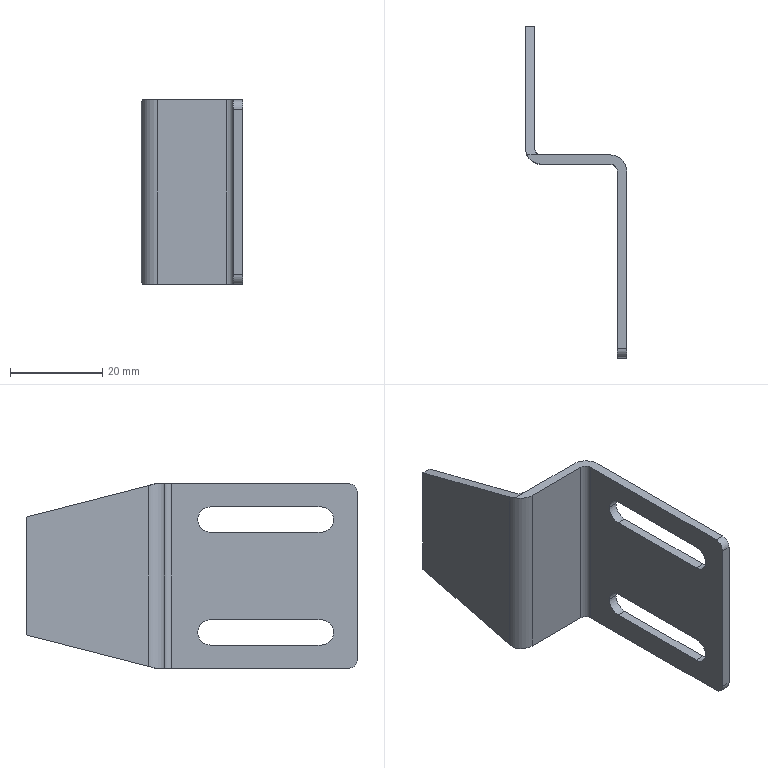Part | NX | features BREP 1 | 1 solid | 28 faces | box 22 x 72 x 40 mm | volume 6159 mm3 | plane 16 | cylinder 12 | commonest cylinder face diameters 5.5 x6 3 x2 4 x2 7 x2
STEP:
#1=CARTESIAN_POINT('',(0.,-7.25,-12.25));
#2=VERTEX_POINT('',#1);
#3=CARTESIAN_POINT('',(0.,-10.,-9.5));
#4=VERTEX_POINT('',#3);
#5=CARTESIAN_POINT('',(0.,-10.,-12.25));
#6=DIRECTION('',(1.,0.,0.));
#7=DIRECTION('',(0.,1.,0.));
#8=AXIS2_PLACEMENT_3D('',#5,#6,#7);
#9=CIRCLE('',#8,2.75);
#10=EDGE_CURVE('',#2,#4,#9,.T.);
#11=ORIENTED_EDGE('',*,*,#10,.F.);
#12=CARTESIAN_POINT('',(2.,-7.25,-12.25));
#13=VERTEX_POINT('',#12);
#14=CARTESIAN_POINT('',(-20.,-7.25,-12.25));
#15=DIRECTION('',(1.,0.,0.));
#16=VECTOR('',#15,1000.);
#17=LINE('',#14,#16);
#18=EDGE_CURVE('',#2,#13,#17,.T.);
#19=ORIENTED_EDGE('',*,*,#18,.T.);
#20=CARTESIAN_POINT('',(2.,-10.,-9.5));
#21=VERTEX_POINT('',#20);
#22=CARTESIAN_POINT('',(2.,-10.,-12.25));
#23=DIRECTION('',(1.,0.,0.));
#24=DIRECTION('',(0.,-1.,0.));
#25=AXIS2_PLACEMENT_3D('',#22,#23,#24);
#26=CIRCLE('',#25,2.75);
#27=EDGE_CURVE('',#13,#21,#26,.T.);
#28=ORIENTED_EDGE('',*,*,#27,.T.);
#29=CARTESIAN_POINT('',(-20.,-10.,-9.5));
#30=DIRECTION('',(1.,0.,0.));
#31=VECTOR('',#30,1000.);
#32=LINE('',#29,#31);
#33=EDGE_CURVE('',#4,#21,#32,.T.);
#34=ORIENTED_EDGE('',*,*,#33,.F.);
#35=EDGE_LOOP('',(#11,#19,#28,#34));
#36=FACE_BOUND('',#35,.T.);
#37=CARTESIAN_POINT('',(-20.,-10.,-12.25));
#38=DIRECTION('',(1.,0.,0.));
#39=DIRECTION('',(0.,1.,0.));
#40=AXIS2_PLACEMENT_3D('',#37,#38,#39);
#41=CYLINDRICAL_SURFACE('',#40,2.75);
#42=ADVANCED_FACE('',(#36),#41,.F.);
#43=CARTESIAN_POINT('',(0.,-7.25,12.25));
#44=VERTEX_POINT('',#43);
#45=CARTESIAN_POINT('',(0.,-10.,15.));
#46=VERTEX_POINT('',#45);
#47=CARTESIAN_POINT('',(0.,-10.,12.25));
#48=DIRECTION('',(1.,0.,0.));
#49=DIRECTION('',(0.,1.,0.));
#50=AXIS2_PLACEMENT_3D('',#47,#48,#49);
#51=CIRCLE('',#50,2.75);
#52=EDGE_CURVE('',#44,#46,#51,.T.);
#53=ORIENTED_EDGE('',*,*,#52,.F.);
#54=CARTESIAN_POINT('',(2.,-7.25,12.25));
#55=VERTEX_POINT('',#54);
#56=CARTESIAN_POINT('',(-20.,-7.25,12.25));
#57=DIRECTION('',(1.,0.,0.));
#58=VECTOR('',#57,1000.);
#59=LINE('',#56,#58);
#60=EDGE_CURVE('',#44,#55,#59,.T.);
#61=ORIENTED_EDGE('',*,*,#60,.T.);
#62=CARTESIAN_POINT('',(2.,-10.,15.));
#63=VERTEX_POINT('',#62);
#64=CARTESIAN_POINT('',(2.,-10.,12.25));
#65=DIRECTION('',(1.,0.,0.));
#66=DIRECTION('',(0.,1.,0.));
#67=AXIS2_PLACEMENT_3D('',#64,#65,#66);
#68=CIRCLE('',#67,2.75);
#69=EDGE_CURVE('',#55,#63,#68,.T.);
#70=ORIENTED_EDGE('',*,*,#69,.T.);
#71=CARTESIAN_POINT('',(-20.,-10.,15.));
#72=DIRECTION('',(1.,0.,0.));
#73=VECTOR('',#72,1000.);
#74=LINE('',#71,#73);
#75=EDGE_CURVE('',#46,#63,#74,.T.);
#76=ORIENTED_EDGE('',*,*,#75,.F.);
#77=EDGE_LOOP('',(#53,#61,#70,#76));
#78=FACE_BOUND('',#77,.T.);
#79=CARTESIAN_POINT('',(-20.,-10.,12.25));
#80=DIRECTION('',(1.,0.,0.));
#81=DIRECTION('',(0.,1.,0.));
#82=AXIS2_PLACEMENT_3D('',#79,#80,#81);
#83=CYLINDRICAL_SURFACE('',#82,2.75);
#84=ADVANCED_FACE('',(#78),#83,.F.);
#85=CARTESIAN_POINT('',(2.,-42.,18.));
#86=VERTEX_POINT('',#85);
#87=CARTESIAN_POINT('',(2.,-42.,-18.));
#88=VERTEX_POINT('',#87);
#89=CARTESIAN_POINT('',(2.,-42.,20.));
#90=DIRECTION('',(0.,0.,-1.));
#91=VECTOR('',#90,1000.);
#92=LINE('',#89,#91);
#93=EDGE_CURVE('',#86,#88,#92,.T.);
#94=ORIENTED_EDGE('',*,*,#93,.T.);
#95=CARTESIAN_POINT('',(2.,-40.,-20.));
#96=VERTEX_POINT('',#95);
#97=CARTESIAN_POINT('',(2.,-40.,-18.));
#98=DIRECTION('',(1.,0.,0.));
#99=DIRECTION('',(0.,-1.,0.));
#100=AXIS2_PLACEMENT_3D('',#97,#98,#99);
#101=CIRCLE('',#100,2.);
#102=EDGE_CURVE('',#88,#96,#101,.T.);
#103=ORIENTED_EDGE('',*,*,#102,.T.);
#104=CARTESIAN_POINT('',(2.,-1.5,-20.));
#105=VERTEX_POINT('',#104);
#106=CARTESIAN_POINT('',(2.,2.,-20.));
#107=DIRECTION('',(0.,1.,0.));
#108=VECTOR('',#107,1000.);
#109=LINE('',#106,#108);
#110=EDGE_CURVE('',#96,#105,#109,.T.);
#111=ORIENTED_EDGE('',*,*,#110,.T.);
#112=CARTESIAN_POINT('',(2.,-1.5,20.));
#113=VERTEX_POINT('',#112);
#114=CARTESIAN_POINT('',(2.,-1.5,20.));
#115=DIRECTION('',(0.,0.,1.));
#116=VECTOR('',#115,1000.);
#117=LINE('',#114,#116);
#118=EDGE_CURVE('',#105,#113,#117,.T.);
#119=ORIENTED_EDGE('',*,*,#118,.T.);
#120=CARTESIAN_POINT('',(2.,-40.,20.));
#121=VERTEX_POINT('',#120);
#122=CARTESIAN_POINT('',(2.,2.,20.));
#123=DIRECTION('',(0.,1.,0.));
#124=VECTOR('',#123,1000.);
#125=LINE('',#122,#124);
#126=EDGE_CURVE('',#121,#113,#125,.T.);
#127=ORIENTED_EDGE('',*,*,#126,.F.);
#128=CARTESIAN_POINT('',(2.,-40.,18.));
#129=DIRECTION('',(1.,0.,0.));
#130=DIRECTION('',(0.,-1.,0.));
#131=AXIS2_PLACEMENT_3D('',#128,#129,#130);
#132=CIRCLE('',#131,2.);
#133=EDGE_CURVE('',#121,#86,#132,.T.);
#134=ORIENTED_EDGE('',*,*,#133,.T.);
#135=EDGE_LOOP('',(#94,#103,#111,#119,#127,#134));
#136=FACE_BOUND('',#135,.T.);
#137=CARTESIAN_POINT('',(2.,-34.,-9.5));
#138=VERTEX_POINT('',#137);
#139=CARTESIAN_POINT('',(2.,-10.,-9.5));
#140=DIRECTION('',(0.,-1.,0.));
#141=VECTOR('',#140,1000.);
#142=LINE('',#139,#141);
#143=EDGE_CURVE('',#21,#138,#142,.T.);
#144=ORIENTED_EDGE('',*,*,#143,.F.);
#145=ORIENTED_EDGE('',*,*,#27,.F.);
#146=CARTESIAN_POINT('',(2.,-10.,-15.));
#147=VERTEX_POINT('',#146);
#148=CARTESIAN_POINT('',(2.,-10.,-12.25));
#149=DIRECTION('',(1.,0.,0.));
#150=DIRECTION('',(0.,-1.,0.));
#151=AXIS2_PLACEMENT_3D('',#148,#149,#150);
#152=CIRCLE('',#151,2.75);
#153=EDGE_CURVE('',#147,#13,#152,.T.);
#154=ORIENTED_EDGE('',*,*,#153,.F.);
#155=CARTESIAN_POINT('',(2.,-34.,-15.));
#156=VERTEX_POINT('',#155);
#157=CARTESIAN_POINT('',(2.,-10.,-15.));
#158=DIRECTION('',(0.,1.,0.));
#159=VECTOR('',#158,1000.);
#160=LINE('',#157,#159);
#161=EDGE_CURVE('',#156,#147,#160,.T.);
#162=ORIENTED_EDGE('',*,*,#161,.F.);
#163=CARTESIAN_POINT('',(2.,-34.,-12.25));
#164=DIRECTION('',(1.,0.,0.));
#165=DIRECTION('',(0.,-1.,0.));
#166=AXIS2_PLACEMENT_3D('',#163,#164,#165);
#167=CIRCLE('',#166,2.75);
#168=EDGE_CURVE('',#138,#156,#167,.T.);
#169=ORIENTED_EDGE('',*,*,#168,.F.);
#170=EDGE_LOOP('',(#144,#145,#154,#162,#169));
#171=FACE_BOUND('',#170,.T.);
#172=CARTESIAN_POINT('',(2.,-34.,15.));
#173=VERTEX_POINT('',#172);
#174=CARTESIAN_POINT('',(2.,-10.,15.));
#175=DIRECTION('',(0.,-1.,0.));
#176=VECTOR('',#175,1000.);
#177=LINE('',#174,#176);
#178=EDGE_CURVE('',#63,#173,#177,.T.);
#179=ORIENTED_EDGE('',*,*,#178,.F.);
#180=ORIENTED_EDGE('',*,*,#69,.F.);
#181=CARTESIAN_POINT('',(2.,-10.,9.5));
#182=VERTEX_POINT('',#181);
#183=CARTESIAN_POINT('',(2.,-10.,12.25));
#184=DIRECTION('',(1.,0.,0.));
#185=DIRECTION('',(0.,1.,0.));
#186=AXIS2_PLACEMENT_3D('',#183,#184,#185);
#187=CIRCLE('',#186,2.75);
#188=EDGE_CURVE('',#182,#55,#187,.T.);
#189=ORIENTED_EDGE('',*,*,#188,.F.);
#190=CARTESIAN_POINT('',(2.,-34.,9.5));
#191=VERTEX_POINT('',#190);
#192=CARTESIAN_POINT('',(2.,-10.,9.5));
#193=DIRECTION('',(0.,1.,0.));
#194=VECTOR('',#193,1000.);
#195=LINE('',#192,#194);
#196=EDGE_CURVE('',#191,#182,#195,.T.);
#197=ORIENTED_EDGE('',*,*,#196,.F.);
#198=CARTESIAN_POINT('',(2.,-34.,12.25));
#199=DIRECTION('',(1.,0.,0.));
#200=DIRECTION('',(0.,1.,0.));
#201=AXIS2_PLACEMENT_3D('',#198,#199,#200);
#202=CIRCLE('',#201,2.75);
#203=EDGE_CURVE('',#173,#191,#202,.T.);
#204=ORIENTED_EDGE('',*,*,#203,.F.);
#205=EDGE_LOOP('',(#179,#180,#189,#197,#204));
#206=FACE_BOUND('',#205,.T.);
#207=CARTESIAN_POINT('',(2.,2.,20.));
#208=DIRECTION('',(-1.,0.,0.));
#209=DIRECTION('',(0.,1.,0.));
#210=AXIS2_PLACEMENT_3D('',#207,#208,#209);
#211=PLANE('',#210);
#212=ADVANCED_FACE('',(#136,#171,#206),#211,.F.);
#213=CARTESIAN_POINT('',(-1.5,2.,20.));
#214=VERTEX_POINT('',#213);
#215=CARTESIAN_POINT('',(-16.5,2.,20.));
#216=VERTEX_POINT('',#215);
#217=CARTESIAN_POINT('',(-18.,2.,20.));
#218=DIRECTION('',(-1.,0.,0.));
#219=VECTOR('',#218,1000.);
#220=LINE('',#217,#219);
#221=EDGE_CURVE('',#214,#216,#220,.T.);
#222=ORIENTED_EDGE('',*,*,#221,.F.);
#223=CARTESIAN_POINT('',(-1.5,2.,-20.));
#224=VERTEX_POINT('',#223);
#225=CARTESIAN_POINT('',(-1.5,2.,20.));
#226=DIRECTION('',(0.,0.,-1.));
#227=VECTOR('',#226,1000.);
#228=LINE('',#225,#227);
#229=EDGE_CURVE('',#214,#224,#228,.T.);
#230=ORIENTED_EDGE('',*,*,#229,.T.);
#231=CARTESIAN_POINT('',(-16.5,2.,-20.));
#232=VERTEX_POINT('',#231);
#233=CARTESIAN_POINT('',(-18.,2.,-20.));
#234=DIRECTION('',(-1.,0.,0.));
#235=VECTOR('',#234,1000.);
#236=LINE('',#233,#235);
#237=EDGE_CURVE('',#224,#232,#236,.T.);
#238=ORIENTED_EDGE('',*,*,#237,.T.);
#239=CARTESIAN_POINT('',(-16.5,2.,20.));
#240=DIRECTION('',(0.,0.,1.));
#241=VECTOR('',#240,1000.);
#242=LINE('',#239,#241);
#243=EDGE_CURVE('',#232,#216,#242,.T.);
#244=ORIENTED_EDGE('',*,*,#243,.T.);
#245=EDGE_LOOP('',(#222,#230,#238,#244));
#246=FACE_BOUND('',#245,.T.);
#247=CARTESIAN_POINT('',(-18.,2.,20.));
#248=DIRECTION('',(0.,-1.,0.));
#249=DIRECTION('',(-1.,0.,0.));
#250=AXIS2_PLACEMENT_3D('',#247,#248,#249);
#251=PLANE('',#250);
#252=ADVANCED_FACE('',(#246),#251,.F.);
#253=CARTESIAN_POINT('',(-18.,30.,12.8));
#254=VERTEX_POINT('',#253);
#255=CARTESIAN_POINT('',(-18.,3.5,19.614));
#256=VERTEX_POINT('',#255);
#257=CARTESIAN_POINT('',(-18.,28.263,13.247));
#258=DIRECTION('',(0.,-0.9685,0.249));
#259=VECTOR('',#258,1000.);
#260=LINE('',#257,#259);
#261=EDGE_CURVE('',#254,#256,#260,.T.);
#262=ORIENTED_EDGE('',*,*,#261,.T.);
#263=CARTESIAN_POINT('',(-18.,3.5,-19.614));
#264=VERTEX_POINT('',#263);
#265=CARTESIAN_POINT('',(-18.,3.5,-20.));
#266=DIRECTION('',(0.,0.,-1.));
#267=VECTOR('',#266,1000.);
#268=LINE('',#265,#267);
#269=EDGE_CURVE('',#256,#264,#268,.T.);
#270=ORIENTED_EDGE('',*,*,#269,.T.);
#271=CARTESIAN_POINT('',(-18.,30.,-12.8));
#272=VERTEX_POINT('',#271);
#273=CARTESIAN_POINT('',(-18.,37.911,-10.766));
#274=DIRECTION('',(0.,0.9685,0.249));
#275=VECTOR('',#274,1000.);
#276=LINE('',#273,#275);
#277=EDGE_CURVE('',#264,#272,#276,.T.);
#278=ORIENTED_EDGE('',*,*,#277,.T.);
#279=CARTESIAN_POINT('',(-18.,30.,20.));
#280=DIRECTION('',(0.,0.,-1.));
#281=VECTOR('',#280,1000.);
#282=LINE('',#279,#281);
#283=EDGE_CURVE('',#254,#272,#282,.T.);
#284=ORIENTED_EDGE('',*,*,#283,.F.);
#285=EDGE_LOOP('',(#262,#270,#278,#284));
#286=FACE_BOUND('',#285,.T.);
#287=CARTESIAN_POINT('',(-18.,30.,20.));
#288=DIRECTION('',(-1.,0.,0.));
#289=DIRECTION('',(0.,1.,0.));
#290=AXIS2_PLACEMENT_3D('',#287,#288,#289);
#291=PLANE('',#290);
#292=ADVANCED_FACE('',(#286),#291,.F.);
#293=ORIENTED_EDGE('',*,*,#283,.T.);
#294=CARTESIAN_POINT('',(-20.,30.,-12.8));
#295=VERTEX_POINT('',#294);
#296=CARTESIAN_POINT('',(-20.,30.,-12.8));
#297=DIRECTION('',(1.,0.,0.));
#298=VECTOR('',#297,1000.);
#299=LINE('',#296,#298);
#300=EDGE_CURVE('',#295,#272,#299,.T.);
#301=ORIENTED_EDGE('',*,*,#300,.F.);
#302=CARTESIAN_POINT('',(-20.,30.,12.8));
#303=VERTEX_POINT('',#302);
#304=CARTESIAN_POINT('',(-20.,30.,20.));
#305=DIRECTION('',(0.,0.,-1.));
#306=VECTOR('',#305,1000.);
#307=LINE('',#304,#306);
#308=EDGE_CURVE('',#303,#295,#307,.T.);
#309=ORIENTED_EDGE('',*,*,#308,.F.);
#310=CARTESIAN_POINT('',(-20.,30.,12.8));
#311=DIRECTION('',(1.,0.,0.));
#312=VECTOR('',#311,1000.);
#313=LINE('',#310,#312);
#314=EDGE_CURVE('',#303,#254,#313,.T.);
#315=ORIENTED_EDGE('',*,*,#314,.T.);
#316=EDGE_LOOP('',(#293,#301,#309,#315));
#317=FACE_BOUND('',#316,.T.);
#318=CARTESIAN_POINT('',(-20.,30.,20.));
#319=DIRECTION('',(0.,-1.,0.));
#320=DIRECTION('',(0.,0.,-1.));
#321=AXIS2_PLACEMENT_3D('',#318,#319,#320);
#322=PLANE('',#321);
#323=ADVANCED_FACE('',(#317),#322,.F.);
#324=CARTESIAN_POINT('',(-20.,3.5,-19.614));
#325=VERTEX_POINT('',#324);
#326=CARTESIAN_POINT('',(-20.,30.,-12.8));
#327=DIRECTION('',(0.,-0.9685,-0.249));
#328=VECTOR('',#327,1000.);
#329=LINE('',#326,#328);
#330=EDGE_CURVE('',#295,#325,#329,.T.);
#331=ORIENTED_EDGE('',*,*,#330,.T.);
#332=CARTESIAN_POINT('',(-20.,3.5,19.614));
#333=VERTEX_POINT('',#332);
#334=CARTESIAN_POINT('',(-20.,3.5,20.));
#335=DIRECTION('',(0.,0.,1.));
#336=VECTOR('',#335,1000.);
#337=LINE('',#334,#336);
#338=EDGE_CURVE('',#325,#333,#337,.T.);
#339=ORIENTED_EDGE('',*,*,#338,.T.);
#340=CARTESIAN_POINT('',(-20.,30.,12.8));
#341=DIRECTION('',(0.,0.9685,-0.249));
#342=VECTOR('',#341,1000.);
#343=LINE('',#340,#342);
#344=EDGE_CURVE('',#333,#303,#343,.T.);
#345=ORIENTED_EDGE('',*,*,#344,.T.);
#346=ORIENTED_EDGE('',*,*,#308,.T.);
#347=EDGE_LOOP('',(#331,#339,#345,#346));
#348=FACE_BOUND('',#347,.T.);
#349=CARTESIAN_POINT('',(-20.,0.,20.));
#350=DIRECTION('',(1.,0.,0.));
#351=DIRECTION('',(0.,1.,0.));
#352=AXIS2_PLACEMENT_3D('',#349,#350,#351);
#353=PLANE('',#352);
#354=ADVANCED_FACE('',(#348),#353,.F.);
#355=CARTESIAN_POINT('',(-16.5,0.,20.));
#356=VERTEX_POINT('',#355);
#357=CARTESIAN_POINT('',(-1.5,0.,20.));
#358=VERTEX_POINT('',#357);
#359=CARTESIAN_POINT('',(0.,0.,20.));
#360=DIRECTION('',(1.,0.,0.));
#361=VECTOR('',#360,1000.);
#362=LINE('',#359,#361);
#363=EDGE_CURVE('',#356,#358,#362,.T.);
#364=ORIENTED_EDGE('',*,*,#363,.F.);
#365=CARTESIAN_POINT('',(-16.5,0.,-20.));
#366=VERTEX_POINT('',#365);
#367=CARTESIAN_POINT('',(-16.5,0.,20.));
#368=DIRECTION('',(0.,0.,-1.));
#369=VECTOR('',#368,1000.);
#370=LINE('',#367,#369);
#371=EDGE_CURVE('',#356,#366,#370,.T.);
#372=ORIENTED_EDGE('',*,*,#371,.T.);
#373=CARTESIAN_POINT('',(-1.5,0.,-20.));
#374=VERTEX_POINT('',#373);
#375=CARTESIAN_POINT('',(0.,0.,-20.));
#376=DIRECTION('',(1.,0.,0.));
#377=VECTOR('',#376,1000.);
#378=LINE('',#375,#377);
#379=EDGE_CURVE('',#366,#374,#378,.T.);
#380=ORIENTED_EDGE('',*,*,#379,.T.);
#381=CARTESIAN_POINT('',(-1.5,0.,20.));
#382=DIRECTION('',(0.,0.,1.));
#383=VECTOR('',#382,1000.);
#384=LINE('',#381,#383);
#385=EDGE_CURVE('',#374,#358,#384,.T.);
#386=ORIENTED_EDGE('',*,*,#385,.T.);
#387=EDGE_LOOP('',(#364,#372,#380,#386));
#388=FACE_BOUND('',#387,.T.);
#389=CARTESIAN_POINT('',(0.,0.,20.));
#390=DIRECTION('',(0.,1.,0.));
#391=DIRECTION('',(1.,0.,0.));
#392=AXIS2_PLACEMENT_3D('',#389,#390,#391);
#393=PLANE('',#392);
#394=ADVANCED_FACE('',(#388),#393,.F.);
#395=CARTESIAN_POINT('',(0.,-1.5,-20.));
#396=VERTEX_POINT('',#395);
#397=CARTESIAN_POINT('',(0.,-40.,-20.));
#398=VERTEX_POINT('',#397);
#399=CARTESIAN_POINT('',(0.,-42.,-20.));
#400=DIRECTION('',(0.,-1.,0.));
#401=VECTOR('',#400,1000.);
#402=LINE('',#399,#401);
#403=EDGE_CURVE('',#396,#398,#402,.T.);
#404=ORIENTED_EDGE('',*,*,#403,.T.);
#405=CARTESIAN_POINT('',(0.,-42.,-18.));
#406=VERTEX_POINT('',#405);
#407=CARTESIAN_POINT('',(0.,-40.,-18.));
#408=DIRECTION('',(-1.,0.,0.));
#409=DIRECTION('',(0.,1.,0.));
#410=AXIS2_PLACEMENT_3D('',#407,#408,#409);
#411=CIRCLE('',#410,2.);
#412=EDGE_CURVE('',#398,#406,#411,.T.);
#413=ORIENTED_EDGE('',*,*,#412,.T.);
#414=CARTESIAN_POINT('',(0.,-42.,18.));
#415=VERTEX_POINT('',#414);
#416=CARTESIAN_POINT('',(0.,-42.,20.));
#417=DIRECTION('',(0.,0.,-1.));
#418=VECTOR('',#417,1000.);
#419=LINE('',#416,#418);
#420=EDGE_CURVE('',#415,#406,#419,.T.);
#421=ORIENTED_EDGE('',*,*,#420,.F.);
#422=CARTESIAN_POINT('',(0.,-40.,20.));
#423=VERTEX_POINT('',#422);
#424=CARTESIAN_POINT('',(0.,-40.,18.));
#425=DIRECTION('',(-1.,0.,0.));
#426=DIRECTION('',(0.,1.,0.));
#427=AXIS2_PLACEMENT_3D('',#424,#425,#426);
#428=CIRCLE('',#427,2.);
#429=EDGE_CURVE('',#415,#423,#428,.T.);
#430=ORIENTED_EDGE('',*,*,#429,.T.);
#431=CARTESIAN_POINT('',(0.,-1.5,20.));
#432=VERTEX_POINT('',#431);
#433=CARTESIAN_POINT('',(0.,-42.,20.));
#434=DIRECTION('',(0.,-1.,0.));
#435=VECTOR('',#434,1000.);
#436=LINE('',#433,#435);
#437=EDGE_CURVE('',#432,#423,#436,.T.);
#438=ORIENTED_EDGE('',*,*,#437,.F.);
#439=CARTESIAN_POINT('',(0.,-1.5,-20.));
#440=DIRECTION('',(0.,0.,-1.));
#441=VECTOR('',#440,1000.);
#442=LINE('',#439,#441);
#443=EDGE_CURVE('',#432,#396,#442,.T.);
#444=ORIENTED_EDGE('',*,*,#443,.T.);
#445=EDGE_LOOP('',(#404,#413,#421,#430,#438,#444));
#446=FACE_BOUND('',#445,.T.);
#447=CARTESIAN_POINT('',(0.,-34.,-15.));
#448=VERTEX_POINT('',#447);
#449=CARTESIAN_POINT('',(0.,-10.,-15.));
#450=VERTEX_POINT('',#449);
#451=CARTESIAN_POINT('',(0.,-42.,-15.));
#452=DIRECTION('',(0.,1.,0.));
#453=VECTOR('',#452,1000.);
#454=LINE('',#451,#453);
#455=EDGE_CURVE('',#448,#450,#454,.T.);
#456=ORIENTED_EDGE('',*,*,#455,.T.);
#457=CARTESIAN_POINT('',(0.,-10.,-12.25));
#458=DIRECTION('',(1.,0.,0.));
#459=DIRECTION('',(0.,1.,0.));
#460=AXIS2_PLACEMENT_3D('',#457,#458,#459);
#461=CIRCLE('',#460,2.75);
#462=EDGE_CURVE('',#450,#2,#461,.T.);
#463=ORIENTED_EDGE('',*,*,#462,.T.);
#464=ORIENTED_EDGE('',*,*,#10,.T.);
#465=CARTESIAN_POINT('',(0.,-34.,-9.5));
#466=VERTEX_POINT('',#465);
#467=CARTESIAN_POINT('',(0.,-42.,-9.5));
#468=DIRECTION('',(0.,-1.,0.));
#469=VECTOR('',#468,1000.);
#470=LINE('',#467,#469);
#471=EDGE_CURVE('',#4,#466,#470,.T.);
#472=ORIENTED_EDGE('',*,*,#471,.T.);
#473=CARTESIAN_POINT('',(0.,-34.,-12.25));
#474=DIRECTION('',(1.,0.,0.));
#475=DIRECTION('',(0.,1.,0.));
#476=AXIS2_PLACEMENT_3D('',#473,#474,#475);
#477=CIRCLE('',#476,2.75);
#478=EDGE_CURVE('',#466,#448,#477,.T.);
#479=ORIENTED_EDGE('',*,*,#478,.T.);
#480=EDGE_LOOP('',(#456,#463,#464,#472,#479));
#481=FACE_BOUND('',#480,.T.);
#482=CARTESIAN_POINT('',(0.,-34.,9.5));
#483=VERTEX_POINT('',#482);
#484=CARTESIAN_POINT('',(0.,-10.,9.5));
#485=VERTEX_POINT('',#484);
#486=CARTESIAN_POINT('',(0.,-42.,9.5));
#487=DIRECTION('',(0.,1.,0.));
#488=VECTOR('',#487,1000.);
#489=LINE('',#486,#488);
#490=EDGE_CURVE('',#483,#485,#489,.T.);
#491=ORIENTED_EDGE('',*,*,#490,.T.);
#492=CARTESIAN_POINT('',(0.,-10.,12.25));
#493=DIRECTION('',(1.,0.,0.));
#494=DIRECTION('',(0.,1.,0.));
#495=AXIS2_PLACEMENT_3D('',#492,#493,#494);
#496=CIRCLE('',#495,2.75);
#497=EDGE_CURVE('',#485,#44,#496,.T.);
#498=ORIENTED_EDGE('',*,*,#497,.T.);
#499=ORIENTED_EDGE('',*,*,#52,.T.);
#500=CARTESIAN_POINT('',(0.,-34.,15.));
#501=VERTEX_POINT('',#500);
#502=CARTESIAN_POINT('',(0.,-42.,15.));
#503=DIRECTION('',(0.,-1.,0.));
#504=VECTOR('',#503,1000.);
#505=LINE('',#502,#504);
#506=EDGE_CURVE('',#46,#501,#505,.T.);
#507=ORIENTED_EDGE('',*,*,#506,.T.);
#508=CARTESIAN_POINT('',(0.,-34.,12.25));
#509=DIRECTION('',(1.,0.,0.));
#510=DIRECTION('',(0.,1.,0.));
#511=AXIS2_PLACEMENT_3D('',#508,#509,#510);
#512=CIRCLE('',#511,2.75);
#513=EDGE_CURVE('',#501,#483,#512,.T.);
#514=ORIENTED_EDGE('',*,*,#513,.T.);
#515=EDGE_LOOP('',(#491,#498,#499,#507,#514));
#516=FACE_BOUND('',#515,.T.);
#517=CARTESIAN_POINT('',(0.,-42.,20.));
#518=DIRECTION('',(1.,0.,0.));
#519=DIRECTION('',(0.,1.,0.));
#520=AXIS2_PLACEMENT_3D('',#517,#518,#519);
#521=PLANE('',#520);
#522=ADVANCED_FACE('',(#446,#481,#516),#521,.F.);
#523=ORIENTED_EDGE('',*,*,#420,.T.);
#524=CARTESIAN_POINT('',(2.,-42.,-18.));
#525=DIRECTION('',(1.,0.,0.));
#526=VECTOR('',#525,1000.);
#527=LINE('',#524,#526);
#528=EDGE_CURVE('',#406,#88,#527,.T.);
#529=ORIENTED_EDGE('',*,*,#528,.T.);
#530=ORIENTED_EDGE('',*,*,#93,.F.);
#531=CARTESIAN_POINT('',(2.,-42.,18.));
#532=DIRECTION('',(-1.,0.,0.));
#533=VECTOR('',#532,1000.);
#534=LINE('',#531,#533);
#535=EDGE_CURVE('',#86,#415,#534,.T.);
#536=ORIENTED_EDGE('',*,*,#535,.T.);
#537=EDGE_LOOP('',(#523,#529,#530,#536));
#538=FACE_BOUND('',#537,.T.);
#539=CARTESIAN_POINT('',(2.,-42.,20.));
#540=DIRECTION('',(0.,1.,0.));
#541=DIRECTION('',(1.,0.,0.));
#542=AXIS2_PLACEMENT_3D('',#539,#540,#541);
#543=PLANE('',#542);
#544=ADVANCED_FACE('',(#538),#543,.F.);
#545=ORIENTED_EDGE('',*,*,#437,.T.);
#546=CARTESIAN_POINT('',(0.,-40.,20.));
#547=DIRECTION('',(1.,0.,0.));
#548=VECTOR('',#547,1000.);
#549=LINE('',#546,#548);
#550=EDGE_CURVE('',#423,#121,#549,.T.);
#551=ORIENTED_EDGE('',*,*,#550,.T.);
#552=ORIENTED_EDGE('',*,*,#126,.T.);
#553=CARTESIAN_POINT('',(-1.5,-1.5,20.));
#554=DIRECTION('',(0.,0.,1.));
#555=DIRECTION('',(-1.,0.,0.));
#556=AXIS2_PLACEMENT_3D('',#553,#554,#555);
#557=CIRCLE('',#556,3.5);
#558=EDGE_CURVE('',#113,#214,#557,.T.);
#559=ORIENTED_EDGE('',*,*,#558,.T.);
#560=ORIENTED_EDGE('',*,*,#221,.T.);
#561=CARTESIAN_POINT('',(-19.662,2.,20.));
#562=VERTEX_POINT('',#561);
#563=CARTESIAN_POINT('',(-20.,2.,20.));
#564=DIRECTION('',(1.,0.,0.));
#565=VECTOR('',#564,1000.);
#566=LINE('',#563,#565);
#567=EDGE_CURVE('',#562,#216,#566,.T.);
#568=ORIENTED_EDGE('',*,*,#567,.F.);
#569=CARTESIAN_POINT('',(-16.5,3.5,20.));
#570=DIRECTION('',(0.,0.,1.));
#571=DIRECTION('',(-1.,0.,0.));
#572=AXIS2_PLACEMENT_3D('',#569,#570,#571);
#573=CIRCLE('',#572,3.5);
#574=EDGE_CURVE('',#562,#356,#573,.T.);
#575=ORIENTED_EDGE('',*,*,#574,.T.);
#576=ORIENTED_EDGE('',*,*,#363,.T.);
#577=CARTESIAN_POINT('',(-1.5,-1.5,20.));
#578=DIRECTION('',(0.,0.,-1.));
#579=DIRECTION('',(-1.,0.,0.));
#580=AXIS2_PLACEMENT_3D('',#577,#578,#579);
#581=CIRCLE('',#580,1.5);
#582=EDGE_CURVE('',#358,#432,#581,.T.);
#583=ORIENTED_EDGE('',*,*,#582,.T.);
#584=EDGE_LOOP('',(#545,#551,#552,#559,#560,#568,#575,#576,#583));
#585=FACE_BOUND('',#584,.T.);
#586=CARTESIAN_POINT('',(0.,0.,20.));
#587=DIRECTION('',(0.,0.,-1.));
#588=DIRECTION('',(0.,-1.,0.));
#589=AXIS2_PLACEMENT_3D('',#586,#587,#588);
#590=PLANE('',#589);
#591=ADVANCED_FACE('',(#585),#590,.F.);
#592=ORIENTED_EDGE('',*,*,#110,.F.);
#593=CARTESIAN_POINT('',(0.,-40.,-20.));
#594=DIRECTION('',(-1.,0.,0.));
#595=VECTOR('',#594,1000.);
#596=LINE('',#593,#595);
#597=EDGE_CURVE('',#96,#398,#596,.T.);
#598=ORIENTED_EDGE('',*,*,#597,.T.);
#599=ORIENTED_EDGE('',*,*,#403,.F.);
#600=CARTESIAN_POINT('',(-1.5,-1.5,-20.));
#601=DIRECTION('',(0.,0.,1.));
#602=DIRECTION('',(-1.,0.,0.));
#603=AXIS2_PLACEMENT_3D('',#600,#601,#602);
#604=CIRCLE('',#603,1.5);
#605=EDGE_CURVE('',#396,#374,#604,.T.);
#606=ORIENTED_EDGE('',*,*,#605,.T.);
#607=ORIENTED_EDGE('',*,*,#379,.F.);
#608=CARTESIAN_POINT('',(-19.662,2.,-20.));
#609=VERTEX_POINT('',#608);
#610=CARTESIAN_POINT('',(-16.5,3.5,-20.));
#611=DIRECTION('',(0.,0.,-1.));
#612=DIRECTION('',(-1.,0.,0.));
#613=AXIS2_PLACEMENT_3D('',#610,#611,#612);
#614=CIRCLE('',#613,3.5);
#615=EDGE_CURVE('',#366,#609,#614,.T.);
#616=ORIENTED_EDGE('',*,*,#615,.T.);
#617=CARTESIAN_POINT('',(-20.,2.,-20.));
#618=DIRECTION('',(1.,0.,0.));
#619=VECTOR('',#618,1000.);
#620=LINE('',#617,#619);
#621=EDGE_CURVE('',#609,#232,#620,.T.);
#622=ORIENTED_EDGE('',*,*,#621,.T.);
#623=ORIENTED_EDGE('',*,*,#237,.F.);
#624=CARTESIAN_POINT('',(-1.5,-1.5,-20.));
#625=DIRECTION('',(0.,0.,-1.));
#626=DIRECTION('',(-1.,0.,0.));
#627=AXIS2_PLACEMENT_3D('',#624,#625,#626);
#628=CIRCLE('',#627,3.5);
#629=EDGE_CURVE('',#224,#105,#628,.T.);
#630=ORIENTED_EDGE('',*,*,#629,.T.);
#631=EDGE_LOOP('',(#592,#598,#599,#606,#607,#616,#622,#623,#630));
#632=FACE_BOUND('',#631,.T.);
#633=CARTESIAN_POINT('',(0.,0.,-20.));
#634=DIRECTION('',(0.,0.,-1.));
#635=DIRECTION('',(0.,-1.,0.));
#636=AXIS2_PLACEMENT_3D('',#633,#634,#635);
#637=PLANE('',#636);
#638=ADVANCED_FACE('',(#632),#637,.T.);
#639=ORIENTED_EDGE('',*,*,#344,.F.);
#640=CARTESIAN_POINT('',(-20.,3.5,19.614));
#641=CARTESIAN_POINT('',(-20.,2.979,19.748));
#642=CARTESIAN_POINT('',(-19.886,2.471,19.879));
#643=CARTESIAN_POINT('',(-19.662,2.,20.));
#644=(BOUNDED_CURVE()B_SPLINE_CURVE(3,(#640,#641,#642,#643),.UNSPECIFIED.,.F.,.F.)B_SPLINE_CURVE_WITH_KNOTS((4,4),(1.571,2.014),.UNSPECIFIED.)CURVE()GEOMETRIC_REPRESENTATION_ITEM()RATIONAL_B_SPLINE_CURVE((1.,0.9837,0.9837,1.))REPRESENTATION_ITEM(''));
#645=EDGE_CURVE('',#333,#562,#644,.T.);
#646=ORIENTED_EDGE('',*,*,#645,.T.);
#647=ORIENTED_EDGE('',*,*,#567,.T.);
#648=CARTESIAN_POINT('',(-16.5,2.,20.));
#649=CARTESIAN_POINT('',(-17.379,2.,20.));
#650=CARTESIAN_POINT('',(-18.,2.621,19.84));
#651=CARTESIAN_POINT('',(-18.,3.5,19.614));
#652=(BOUNDED_CURVE()B_SPLINE_CURVE(3,(#648,#649,#650,#651),.UNSPECIFIED.,.F.,.F.)B_SPLINE_CURVE_WITH_KNOTS((4,4),(0.,1.571),.UNSPECIFIED.)CURVE()GEOMETRIC_REPRESENTATION_ITEM()RATIONAL_B_SPLINE_CURVE((1.,0.8047,0.8047,1.))REPRESENTATION_ITEM(''));
#653=EDGE_CURVE('',#216,#256,#652,.T.);
#654=ORIENTED_EDGE('',*,*,#653,.T.);
#655=ORIENTED_EDGE('',*,*,#261,.F.);
#656=ORIENTED_EDGE('',*,*,#314,.F.);
#657=EDGE_LOOP('',(#639,#646,#647,#654,#655,#656));
#658=FACE_BOUND('',#657,.T.);
#659=CARTESIAN_POINT('',(-20.,30.,12.8));
#660=DIRECTION('',(0.,-0.249,-0.9685));
#661=DIRECTION('',(0.,-0.9685,0.249));
#662=AXIS2_PLACEMENT_3D('',#659,#660,#661);
#663=PLANE('',#662);
#664=ADVANCED_FACE('',(#658),#663,.F.);
#665=ORIENTED_EDGE('',*,*,#621,.F.);
#666=CARTESIAN_POINT('',(-19.662,2.,-20.));
#667=CARTESIAN_POINT('',(-19.886,2.471,-19.879));
#668=CARTESIAN_POINT('',(-20.,2.979,-19.748));
#669=CARTESIAN_POINT('',(-20.,3.5,-19.614));
#670=(BOUNDED_CURVE()B_SPLINE_CURVE(3,(#666,#667,#668,#669),.UNSPECIFIED.,.F.,.F.)B_SPLINE_CURVE_WITH_KNOTS((4,4),(1.128,1.571),.UNSPECIFIED.)CURVE()GEOMETRIC_REPRESENTATION_ITEM()RATIONAL_B_SPLINE_CURVE((1.,0.9837,0.9837,1.))REPRESENTATION_ITEM(''));
#671=EDGE_CURVE('',#609,#325,#670,.T.);
#672=ORIENTED_EDGE('',*,*,#671,.T.);
#673=ORIENTED_EDGE('',*,*,#330,.F.);
#674=ORIENTED_EDGE('',*,*,#300,.T.);
#675=ORIENTED_EDGE('',*,*,#277,.F.);
#676=CARTESIAN_POINT('',(-18.,3.5,-19.614));
#677=CARTESIAN_POINT('',(-18.,2.621,-19.84));
#678=CARTESIAN_POINT('',(-17.379,2.,-20.));
#679=CARTESIAN_POINT('',(-16.5,2.,-20.));
#680=(BOUNDED_CURVE()B_SPLINE_CURVE(3,(#676,#677,#678,#679),.UNSPECIFIED.,.F.,.F.)B_SPLINE_CURVE_WITH_KNOTS((4,4),(1.571,3.142),.UNSPECIFIED.)CURVE()GEOMETRIC_REPRESENTATION_ITEM()RATIONAL_B_SPLINE_CURVE((1.,0.8047,0.8047,1.))REPRESENTATION_ITEM(''));
#681=EDGE_CURVE('',#264,#232,#680,.T.);
#682=ORIENTED_EDGE('',*,*,#681,.T.);
#683=EDGE_LOOP('',(#665,#672,#673,#674,#675,#682));
#684=FACE_BOUND('',#683,.T.);
#685=CARTESIAN_POINT('',(-20.,30.,-12.8));
#686=DIRECTION('',(0.,-0.249,0.9685));
#687=DIRECTION('',(-1.,0.,0.));
#688=AXIS2_PLACEMENT_3D('',#685,#686,#687);
#689=PLANE('',#688);
#690=ADVANCED_FACE('',(#684),#689,.F.);
#691=ORIENTED_EDGE('',*,*,#60,.F.);
#692=ORIENTED_EDGE('',*,*,#497,.F.);
#693=CARTESIAN_POINT('',(-20.,-10.,9.5));
#694=DIRECTION('',(1.,0.,0.));
#695=VECTOR('',#694,1000.);
#696=LINE('',#693,#695);
#697=EDGE_CURVE('',#485,#182,#696,.T.);
#698=ORIENTED_EDGE('',*,*,#697,.T.);
#699=ORIENTED_EDGE('',*,*,#188,.T.);
#700=EDGE_LOOP('',(#691,#692,#698,#699));
#701=FACE_BOUND('',#700,.T.);
#702=CARTESIAN_POINT('',(-20.,-10.,12.25));
#703=DIRECTION('',(1.,0.,0.));
#704=DIRECTION('',(0.,1.,0.));
#705=AXIS2_PLACEMENT_3D('',#702,#703,#704);
#706=CYLINDRICAL_SURFACE('',#705,2.75);
#707=ADVANCED_FACE('',(#701),#706,.F.);
#708=CARTESIAN_POINT('',(-20.,-34.,9.5));
#709=DIRECTION('',(1.,0.,0.));
#710=VECTOR('',#709,1000.);
#711=LINE('',#708,#710);
#712=EDGE_CURVE('',#483,#191,#711,.T.);
#713=ORIENTED_EDGE('',*,*,#712,.T.);
#714=ORIENTED_EDGE('',*,*,#196,.T.);
#715=ORIENTED_EDGE('',*,*,#697,.F.);
#716=ORIENTED_EDGE('',*,*,#490,.F.);
#717=EDGE_LOOP('',(#713,#714,#715,#716));
#718=FACE_BOUND('',#717,.T.);
#719=CARTESIAN_POINT('',(-20.,-10.,9.5));
#720=DIRECTION('',(0.,0.,-1.));
#721=DIRECTION('',(-1.,0.,0.));
#722=AXIS2_PLACEMENT_3D('',#719,#720,#721);
#723=PLANE('',#722);
#724=ADVANCED_FACE('',(#718),#723,.F.);
#725=CARTESIAN_POINT('',(-20.,-34.,15.));
#726=DIRECTION('',(1.,0.,0.));
#727=VECTOR('',#726,1000.);
#728=LINE('',#725,#727);
#729=EDGE_CURVE('',#501,#173,#728,.T.);
#730=ORIENTED_EDGE('',*,*,#729,.T.);
#731=ORIENTED_EDGE('',*,*,#203,.T.);
#732=ORIENTED_EDGE('',*,*,#712,.F.);
#733=ORIENTED_EDGE('',*,*,#513,.F.);
#734=EDGE_LOOP('',(#730,#731,#732,#733));
#735=FACE_BOUND('',#734,.T.);
#736=CARTESIAN_POINT('',(-20.,-34.,12.25));
#737=DIRECTION('',(1.,0.,0.));
#738=DIRECTION('',(0.,1.,0.));
#739=AXIS2_PLACEMENT_3D('',#736,#737,#738);
#740=CYLINDRICAL_SURFACE('',#739,2.75);
#741=ADVANCED_FACE('',(#735),#740,.F.);
#742=ORIENTED_EDGE('',*,*,#75,.T.);
#743=ORIENTED_EDGE('',*,*,#178,.T.);
#744=ORIENTED_EDGE('',*,*,#729,.F.);
#745=ORIENTED_EDGE('',*,*,#506,.F.);
#746=EDGE_LOOP('',(#742,#743,#744,#745));
#747=FACE_BOUND('',#746,.T.);
#748=CARTESIAN_POINT('',(-20.,-10.,15.));
#749=DIRECTION('',(0.,0.,1.));
#750=DIRECTION('',(0.,-1.,0.));
#751=AXIS2_PLACEMENT_3D('',#748,#749,#750);
#752=PLANE('',#751);
#753=ADVANCED_FACE('',(#747),#752,.F.);
#754=ORIENTED_EDGE('',*,*,#18,.F.);
#755=ORIENTED_EDGE('',*,*,#462,.F.);
#756=CARTESIAN_POINT('',(-20.,-10.,-15.));
#757=DIRECTION('',(1.,0.,0.));
#758=VECTOR('',#757,1000.);
#759=LINE('',#756,#758);
#760=EDGE_CURVE('',#450,#147,#759,.T.);
#761=ORIENTED_EDGE('',*,*,#760,.T.);
#762=ORIENTED_EDGE('',*,*,#153,.T.);
#763=EDGE_LOOP('',(#754,#755,#761,#762));
#764=FACE_BOUND('',#763,.T.);
#765=CARTESIAN_POINT('',(-20.,-10.,-12.25));
#766=DIRECTION('',(1.,0.,0.));
#767=DIRECTION('',(0.,1.,0.));
#768=AXIS2_PLACEMENT_3D('',#765,#766,#767);
#769=CYLINDRICAL_SURFACE('',#768,2.75);
#770=ADVANCED_FACE('',(#764),#769,.F.);
#771=CARTESIAN_POINT('',(-20.,-34.,-15.));
#772=DIRECTION('',(1.,0.,0.));
#773=VECTOR('',#772,1000.);
#774=LINE('',#771,#773);
#775=EDGE_CURVE('',#448,#156,#774,.T.);
#776=ORIENTED_EDGE('',*,*,#775,.T.);
#777=ORIENTED_EDGE('',*,*,#161,.T.);
#778=ORIENTED_EDGE('',*,*,#760,.F.);
#779=ORIENTED_EDGE('',*,*,#455,.F.);
#780=EDGE_LOOP('',(#776,#777,#778,#779));
#781=FACE_BOUND('',#780,.T.);
#782=CARTESIAN_POINT('',(-20.,-10.,-15.));
#783=DIRECTION('',(0.,0.,-1.));
#784=DIRECTION('',(-1.,0.,0.));
#785=AXIS2_PLACEMENT_3D('',#782,#783,#784);
#786=PLANE('',#785);
#787=ADVANCED_FACE('',(#781),#786,.F.);
#788=CARTESIAN_POINT('',(-20.,-34.,-9.5));
#789=DIRECTION('',(1.,0.,0.));
#790=VECTOR('',#789,1000.);
#791=LINE('',#788,#790);
#792=EDGE_CURVE('',#466,#138,#791,.T.);
#793=ORIENTED_EDGE('',*,*,#792,.T.);
#794=ORIENTED_EDGE('',*,*,#168,.T.);
#795=ORIENTED_EDGE('',*,*,#775,.F.);
#796=ORIENTED_EDGE('',*,*,#478,.F.);
#797=EDGE_LOOP('',(#793,#794,#795,#796));
#798=FACE_BOUND('',#797,.T.);
#799=CARTESIAN_POINT('',(-20.,-34.,-12.25));
#800=DIRECTION('',(1.,0.,0.));
#801=DIRECTION('',(0.,1.,0.));
#802=AXIS2_PLACEMENT_3D('',#799,#800,#801);
#803=CYLINDRICAL_SURFACE('',#802,2.75);
#804=ADVANCED_FACE('',(#798),#803,.F.);
#805=ORIENTED_EDGE('',*,*,#33,.T.);
#806=ORIENTED_EDGE('',*,*,#143,.T.);
#807=ORIENTED_EDGE('',*,*,#792,.F.);
#808=ORIENTED_EDGE('',*,*,#471,.F.);
#809=EDGE_LOOP('',(#805,#806,#807,#808));
#810=FACE_BOUND('',#809,.T.);
#811=CARTESIAN_POINT('',(-20.,-10.,-9.5));
#812=DIRECTION('',(0.,0.,1.));
#813=DIRECTION('',(0.,-1.,0.));
#814=AXIS2_PLACEMENT_3D('',#811,#812,#813);
#815=PLANE('',#814);
#816=ADVANCED_FACE('',(#810),#815,.F.);
#817=ORIENTED_EDGE('',*,*,#412,.F.);
#818=ORIENTED_EDGE('',*,*,#597,.F.);
#819=ORIENTED_EDGE('',*,*,#102,.F.);
#820=ORIENTED_EDGE('',*,*,#528,.F.);
#821=EDGE_LOOP('',(#817,#818,#819,#820));
#822=FACE_BOUND('',#821,.T.);
#823=CARTESIAN_POINT('',(2.,-40.,-18.));
#824=DIRECTION('',(-1.,0.,0.));
#825=DIRECTION('',(0.,0.,1.));
#826=AXIS2_PLACEMENT_3D('',#823,#824,#825);
#827=CYLINDRICAL_SURFACE('',#826,2.);
#828=ADVANCED_FACE('',(#822),#827,.T.);
#829=ORIENTED_EDGE('',*,*,#429,.F.);
#830=ORIENTED_EDGE('',*,*,#535,.F.);
#831=ORIENTED_EDGE('',*,*,#133,.F.);
#832=ORIENTED_EDGE('',*,*,#550,.F.);
#833=EDGE_LOOP('',(#829,#830,#831,#832));
#834=FACE_BOUND('',#833,.T.);
#835=CARTESIAN_POINT('',(0.,-40.,18.));
#836=DIRECTION('',(1.,0.,0.));
#837=DIRECTION('',(0.,0.,-1.));
#838=AXIS2_PLACEMENT_3D('',#835,#836,#837);
#839=CYLINDRICAL_SURFACE('',#838,2.);
#840=ADVANCED_FACE('',(#834),#839,.T.);
#841=ORIENTED_EDGE('',*,*,#645,.F.);
#842=ORIENTED_EDGE('',*,*,#338,.F.);
#843=ORIENTED_EDGE('',*,*,#671,.F.);
#844=ORIENTED_EDGE('',*,*,#615,.F.);
#845=ORIENTED_EDGE('',*,*,#371,.F.);
#846=ORIENTED_EDGE('',*,*,#574,.F.);
#847=EDGE_LOOP('',(#841,#842,#843,#844,#845,#846));
#848=FACE_BOUND('',#847,.T.);
#849=CARTESIAN_POINT('',(-16.5,3.5,20.));
#850=DIRECTION('',(0.,0.,-1.));
#851=DIRECTION('',(-1.,0.,0.));
#852=AXIS2_PLACEMENT_3D('',#849,#850,#851);
#853=CYLINDRICAL_SURFACE('',#852,3.5);
#854=ADVANCED_FACE('',(#848),#853,.T.);
#855=ORIENTED_EDGE('',*,*,#558,.F.);
#856=ORIENTED_EDGE('',*,*,#118,.F.);
#857=ORIENTED_EDGE('',*,*,#629,.F.);
#858=ORIENTED_EDGE('',*,*,#229,.F.);
#859=EDGE_LOOP('',(#855,#856,#857,#858));
#860=FACE_BOUND('',#859,.T.);
#861=CARTESIAN_POINT('',(-1.5,-1.5,20.));
#862=DIRECTION('',(0.,0.,-1.));
#863=DIRECTION('',(-1.,0.,0.));
#864=AXIS2_PLACEMENT_3D('',#861,#862,#863);
#865=CYLINDRICAL_SURFACE('',#864,3.5);
#866=ADVANCED_FACE('',(#860),#865,.T.);
#867=ORIENTED_EDGE('',*,*,#653,.F.);
#868=ORIENTED_EDGE('',*,*,#243,.F.);
#869=ORIENTED_EDGE('',*,*,#681,.F.);
#870=ORIENTED_EDGE('',*,*,#269,.F.);
#871=EDGE_LOOP('',(#867,#868,#869,#870));
#872=FACE_BOUND('',#871,.T.);
#873=CARTESIAN_POINT('',(-16.5,3.5,20.));
#874=DIRECTION('',(0.,0.,1.));
#875=DIRECTION('',(1.,0.,0.));
#876=AXIS2_PLACEMENT_3D('',#873,#874,#875);
#877=CYLINDRICAL_SURFACE('',#876,1.5);
#878=ADVANCED_FACE('',(#872),#877,.F.);
#879=ORIENTED_EDGE('',*,*,#582,.F.);
#880=ORIENTED_EDGE('',*,*,#385,.F.);
#881=ORIENTED_EDGE('',*,*,#605,.F.);
#882=ORIENTED_EDGE('',*,*,#443,.F.);
#883=EDGE_LOOP('',(#879,#880,#881,#882));
#884=FACE_BOUND('',#883,.T.);
#885=CARTESIAN_POINT('',(-1.5,-1.5,20.));
#886=DIRECTION('',(0.,0.,1.));
#887=DIRECTION('',(1.,0.,0.));
#888=AXIS2_PLACEMENT_3D('',#885,#886,#887);
#889=CYLINDRICAL_SURFACE('',#888,1.5);
#890=ADVANCED_FACE('',(#884),#889,.F.);
#891=CLOSED_SHELL('',(#42,#84,#212,#252,#292,#323,#354,#394,#522,#544,#591,#638,#664,#690,#707,#724,#741,#753,#770,#787,#804,#816,#828,#840,#854,#866,#878,#890));
#892=MANIFOLD_SOLID_BREP('',#891);
#893=(LENGTH_UNIT()NAMED_UNIT(*)SI_UNIT(.MILLI.,.METRE.));
#894=UNCERTAINTY_MEASURE_WITH_UNIT(LENGTH_MEASURE(0.00001),#893,'','');
#895=(NAMED_UNIT(*)PLANE_ANGLE_UNIT()SI_UNIT($,.RADIAN.));
#896=(NAMED_UNIT(*)SI_UNIT($,.STERADIAN.)SOLID_ANGLE_UNIT());
#897=(GEOMETRIC_REPRESENTATION_CONTEXT(3)GLOBAL_UNCERTAINTY_ASSIGNED_CONTEXT((#894))GLOBAL_UNIT_ASSIGNED_CONTEXT((#893,#895,#896))REPRESENTATION_CONTEXT('',''));
#898=ADVANCED_BREP_SHAPE_REPRESENTATION('',(#892),#897);